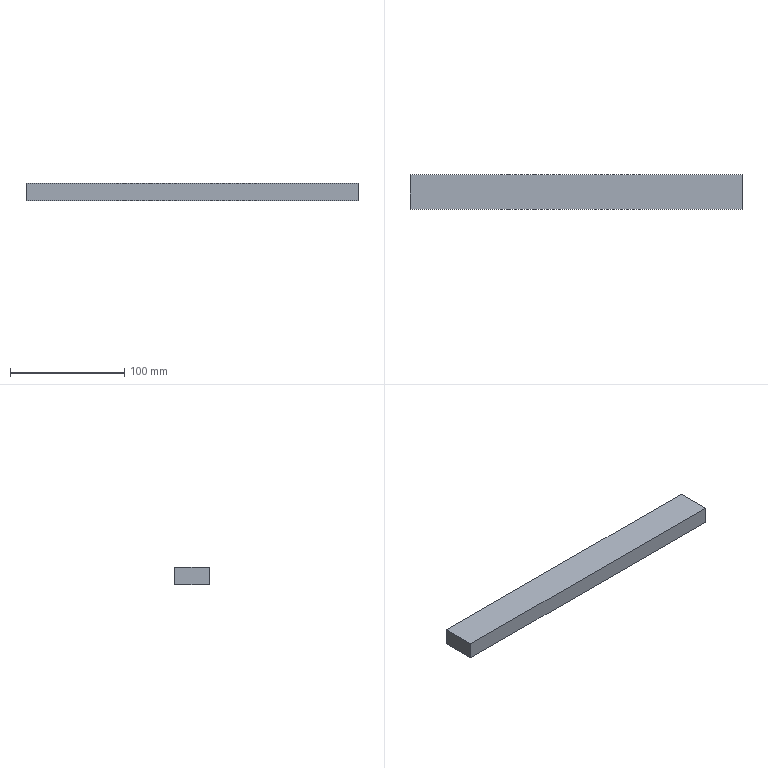Part | NX | features solid 2 | 1 solid | 6 faces | box 290 x 30 x 15 mm | volume 130500 mm3 | plane 6
STEP:
#1=CARTESIAN_POINT('',(157.5,150.,-85.));
#2=VERTEX_POINT('',#1);
#3=CARTESIAN_POINT('',(157.5,120.,-85.));
#4=VERTEX_POINT('',#3);
#5=CARTESIAN_POINT('',(157.5,0.,-85.));
#6=DIRECTION('',(0.,-1.,0.));
#7=VECTOR('',#6,1000.);
#8=LINE('',#5,#7);
#9=EDGE_CURVE('',#2,#4,#8,.T.);
#10=ORIENTED_EDGE('',*,*,#9,.F.);
#11=CARTESIAN_POINT('',(157.5,150.,-100.));
#12=VERTEX_POINT('',#11);
#13=CARTESIAN_POINT('',(157.5,150.,-100.));
#14=DIRECTION('',(0.,0.,-1.));
#15=VECTOR('',#14,1000.);
#16=LINE('',#13,#15);
#17=EDGE_CURVE('',#12,#2,#16,.F.);
#18=ORIENTED_EDGE('',*,*,#17,.F.);
#19=CARTESIAN_POINT('',(157.5,120.,-100.));
#20=VERTEX_POINT('',#19);
#21=CARTESIAN_POINT('',(157.5,0.,-100.));
#22=DIRECTION('',(0.,1.,0.));
#23=VECTOR('',#22,1000.);
#24=LINE('',#21,#23);
#25=EDGE_CURVE('',#12,#20,#24,.F.);
#26=ORIENTED_EDGE('',*,*,#25,.T.);
#27=CARTESIAN_POINT('',(157.5,120.,-100.));
#28=DIRECTION('',(0.,0.,-1.));
#29=VECTOR('',#28,1000.);
#30=LINE('',#27,#29);
#31=EDGE_CURVE('',#20,#4,#30,.F.);
#32=ORIENTED_EDGE('',*,*,#31,.T.);
#33=EDGE_LOOP('',(#10,#18,#26,#32));
#34=FACE_BOUND('',#33,.T.);
#35=CARTESIAN_POINT('',(157.5,0.,-100.));
#36=DIRECTION('',(-1.,0.,0.));
#37=DIRECTION('',(0.,0.,1.));
#38=AXIS2_PLACEMENT_3D('',#35,#36,#37);
#39=PLANE('',#38);
#40=ADVANCED_FACE('',(#34),#39,.T.);
#41=ORIENTED_EDGE('',*,*,#25,.F.);
#42=CARTESIAN_POINT('',(447.5,150.,-100.));
#43=VERTEX_POINT('',#42);
#44=CARTESIAN_POINT('',(177.5,150.,-100.));
#45=DIRECTION('',(1.,0.,0.));
#46=VECTOR('',#45,1000.);
#47=LINE('',#44,#46);
#48=EDGE_CURVE('',#12,#43,#47,.T.);
#49=ORIENTED_EDGE('',*,*,#48,.T.);
#50=CARTESIAN_POINT('',(447.5,120.,-100.));
#51=VERTEX_POINT('',#50);
#52=CARTESIAN_POINT('',(447.5,0.,-100.));
#53=DIRECTION('',(0.,-1.,0.));
#54=VECTOR('',#53,1000.);
#55=LINE('',#52,#54);
#56=EDGE_CURVE('',#43,#51,#55,.T.);
#57=ORIENTED_EDGE('',*,*,#56,.T.);
#58=CARTESIAN_POINT('',(177.5,120.,-100.));
#59=DIRECTION('',(1.,0.,0.));
#60=VECTOR('',#59,1000.);
#61=LINE('',#58,#60);
#62=EDGE_CURVE('',#20,#51,#61,.T.);
#63=ORIENTED_EDGE('',*,*,#62,.F.);
#64=EDGE_LOOP('',(#41,#49,#57,#63));
#65=FACE_BOUND('',#64,.T.);
#66=CARTESIAN_POINT('',(177.5,0.,-100.));
#67=DIRECTION('',(0.,0.,1.));
#68=DIRECTION('',(1.,0.,0.));
#69=AXIS2_PLACEMENT_3D('',#66,#67,#68);
#70=PLANE('',#69);
#71=ADVANCED_FACE('',(#65),#70,.F.);
#72=ORIENTED_EDGE('',*,*,#56,.F.);
#73=CARTESIAN_POINT('',(447.5,150.,-85.));
#74=VERTEX_POINT('',#73);
#75=CARTESIAN_POINT('',(447.5,150.,-85.));
#76=DIRECTION('',(0.,0.,1.));
#77=VECTOR('',#76,1000.);
#78=LINE('',#75,#77);
#79=EDGE_CURVE('',#43,#74,#78,.T.);
#80=ORIENTED_EDGE('',*,*,#79,.T.);
#81=CARTESIAN_POINT('',(447.5,120.,-85.));
#82=VERTEX_POINT('',#81);
#83=CARTESIAN_POINT('',(447.5,0.,-85.));
#84=DIRECTION('',(0.,1.,0.));
#85=VECTOR('',#84,1000.);
#86=LINE('',#83,#85);
#87=EDGE_CURVE('',#74,#82,#86,.F.);
#88=ORIENTED_EDGE('',*,*,#87,.T.);
#89=CARTESIAN_POINT('',(447.5,120.,-85.));
#90=DIRECTION('',(0.,0.,1.));
#91=VECTOR('',#90,1000.);
#92=LINE('',#89,#91);
#93=EDGE_CURVE('',#51,#82,#92,.T.);
#94=ORIENTED_EDGE('',*,*,#93,.F.);
#95=EDGE_LOOP('',(#72,#80,#88,#94));
#96=FACE_BOUND('',#95,.T.);
#97=CARTESIAN_POINT('',(447.5,0.,-85.));
#98=DIRECTION('',(-1.,0.,0.));
#99=DIRECTION('',(0.,0.,1.));
#100=AXIS2_PLACEMENT_3D('',#97,#98,#99);
#101=PLANE('',#100);
#102=ADVANCED_FACE('',(#96),#101,.F.);
#103=CARTESIAN_POINT('',(177.5,150.,-85.));
#104=DIRECTION('',(-1.,0.,0.));
#105=VECTOR('',#104,1000.);
#106=LINE('',#103,#105);
#107=EDGE_CURVE('',#2,#74,#106,.F.);
#108=ORIENTED_EDGE('',*,*,#107,.F.);
#109=ORIENTED_EDGE('',*,*,#9,.T.);
#110=CARTESIAN_POINT('',(177.5,120.,-85.));
#111=DIRECTION('',(-1.,0.,0.));
#112=VECTOR('',#111,1000.);
#113=LINE('',#110,#112);
#114=EDGE_CURVE('',#4,#82,#113,.F.);
#115=ORIENTED_EDGE('',*,*,#114,.T.);
#116=ORIENTED_EDGE('',*,*,#87,.F.);
#117=EDGE_LOOP('',(#108,#109,#115,#116));
#118=FACE_BOUND('',#117,.T.);
#119=CARTESIAN_POINT('',(177.5,0.,-85.));
#120=DIRECTION('',(0.,0.,1.));
#121=DIRECTION('',(1.,0.,0.));
#122=AXIS2_PLACEMENT_3D('',#119,#120,#121);
#123=PLANE('',#122);
#124=ADVANCED_FACE('',(#118),#123,.T.);
#125=ORIENTED_EDGE('',*,*,#93,.T.);
#126=ORIENTED_EDGE('',*,*,#114,.F.);
#127=ORIENTED_EDGE('',*,*,#31,.F.);
#128=ORIENTED_EDGE('',*,*,#62,.T.);
#129=EDGE_LOOP('',(#125,#126,#127,#128));
#130=FACE_BOUND('',#129,.T.);
#131=CARTESIAN_POINT('',(177.5,120.,-100.));
#132=DIRECTION('',(0.,-1.,0.));
#133=DIRECTION('',(0.,0.,-1.));
#134=AXIS2_PLACEMENT_3D('',#131,#132,#133);
#135=PLANE('',#134);
#136=ADVANCED_FACE('',(#130),#135,.T.);
#137=ORIENTED_EDGE('',*,*,#79,.F.);
#138=ORIENTED_EDGE('',*,*,#48,.F.);
#139=ORIENTED_EDGE('',*,*,#17,.T.);
#140=ORIENTED_EDGE('',*,*,#107,.T.);
#141=EDGE_LOOP('',(#137,#138,#139,#140));
#142=FACE_BOUND('',#141,.T.);
#143=CARTESIAN_POINT('',(177.5,150.,-100.));
#144=DIRECTION('',(0.,-1.,0.));
#145=DIRECTION('',(0.,0.,-1.));
#146=AXIS2_PLACEMENT_3D('',#143,#144,#145);
#147=PLANE('',#146);
#148=ADVANCED_FACE('',(#142),#147,.F.);
#149=CLOSED_SHELL('',(#40,#71,#102,#124,#136,#148));
#150=MANIFOLD_SOLID_BREP('',#149);
#151=(LENGTH_UNIT()NAMED_UNIT(*)SI_UNIT(.MILLI.,.METRE.));
#152=UNCERTAINTY_MEASURE_WITH_UNIT(LENGTH_MEASURE(0.00001),#151,'','');
#153=(NAMED_UNIT(*)PLANE_ANGLE_UNIT()SI_UNIT($,.RADIAN.));
#154=(NAMED_UNIT(*)SI_UNIT($,.STERADIAN.)SOLID_ANGLE_UNIT());
#155=(GEOMETRIC_REPRESENTATION_CONTEXT(3)GLOBAL_UNCERTAINTY_ASSIGNED_CONTEXT((#152))GLOBAL_UNIT_ASSIGNED_CONTEXT((#151,#153,#154))REPRESENTATION_CONTEXT('',''));
#156=ADVANCED_BREP_SHAPE_REPRESENTATION('',(#150),#155);